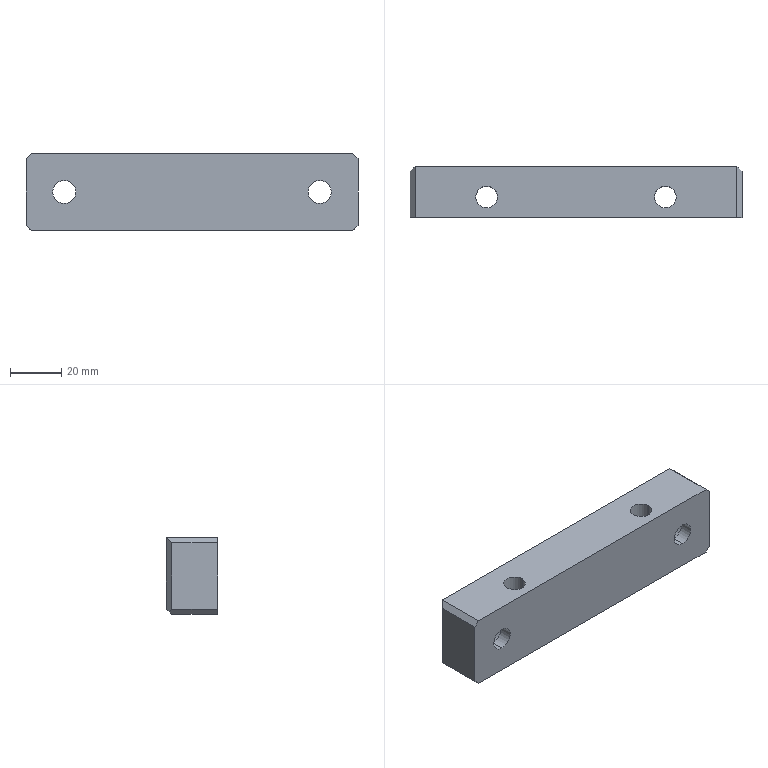Part | SolidWorks | features Chamfer 2, HoleWzd 2, Extrusion 1 | 1 solid | 27 faces | box 130 x 20 x 30 mm | volume 68135 mm3 | plane 15 | cylinder 12 | commonest cylinder face diameters 8.5 x4 9 x4 15 x4
STEP:
#1=CARTESIAN_POINT('',(-39.25,-2.,0.));
#2=VERTEX_POINT('',#1);
#3=CARTESIAN_POINT('',(-30.75,-2.,0.));
#4=VERTEX_POINT('',#3);
#5=CARTESIAN_POINT('',(-35.,-2.,0.));
#6=DIRECTION('',(0.,0.,1.));
#7=DIRECTION('',(1.,0.,0.));
#8=AXIS2_PLACEMENT_3D('',#5,#6,#7);
#9=CIRCLE('',#8,4.25);
#10=EDGE_CURVE('',#2,#4,#9,.T.);
#11=ORIENTED_EDGE('',*,*,#10,.F.);
#12=CARTESIAN_POINT('',(-39.25,-2.,30.));
#13=VERTEX_POINT('',#12);
#14=CARTESIAN_POINT('',(-39.25,-2.,30.));
#15=DIRECTION('',(0.,0.,1.));
#16=VECTOR('',#15,1000.);
#17=LINE('',#14,#16);
#18=EDGE_CURVE('',#2,#13,#17,.T.);
#19=ORIENTED_EDGE('',*,*,#18,.T.);
#20=CARTESIAN_POINT('',(-30.75,-2.,30.));
#21=VERTEX_POINT('',#20);
#22=CARTESIAN_POINT('',(-35.,-2.,30.));
#23=DIRECTION('',(0.,0.,1.));
#24=DIRECTION('',(1.,0.,0.));
#25=AXIS2_PLACEMENT_3D('',#22,#23,#24);
#26=CIRCLE('',#25,4.25);
#27=EDGE_CURVE('',#13,#21,#26,.T.);
#28=ORIENTED_EDGE('',*,*,#27,.T.);
#29=CARTESIAN_POINT('',(-30.75,-2.,30.));
#30=DIRECTION('',(0.,0.,1.));
#31=VECTOR('',#30,1000.);
#32=LINE('',#29,#31);
#33=EDGE_CURVE('',#4,#21,#32,.T.);
#34=ORIENTED_EDGE('',*,*,#33,.F.);
#35=EDGE_LOOP('',(#11,#19,#28,#34));
#36=FACE_OUTER_BOUND('',#35,.T.);
#37=CARTESIAN_POINT('',(-35.,-2.,30.));
#38=DIRECTION('',(0.,0.,1.));
#39=DIRECTION('',(1.,0.,0.));
#40=AXIS2_PLACEMENT_3D('',#37,#38,#39);
#41=CYLINDRICAL_SURFACE('',#40,4.25);
#42=ADVANCED_FACE('',(#36),#41,.F.);
#43=CARTESIAN_POINT('',(30.75,-2.,0.));
#44=VERTEX_POINT('',#43);
#45=CARTESIAN_POINT('',(39.25,-2.,0.));
#46=VERTEX_POINT('',#45);
#47=CARTESIAN_POINT('',(35.,-2.,0.));
#48=DIRECTION('',(0.,0.,1.));
#49=DIRECTION('',(1.,0.,0.));
#50=AXIS2_PLACEMENT_3D('',#47,#48,#49);
#51=CIRCLE('',#50,4.25);
#52=EDGE_CURVE('',#44,#46,#51,.T.);
#53=ORIENTED_EDGE('',*,*,#52,.F.);
#54=CARTESIAN_POINT('',(30.75,-2.,30.));
#55=VERTEX_POINT('',#54);
#56=CARTESIAN_POINT('',(30.75,-2.,30.));
#57=DIRECTION('',(0.,0.,1.));
#58=VECTOR('',#57,1000.);
#59=LINE('',#56,#58);
#60=EDGE_CURVE('',#44,#55,#59,.T.);
#61=ORIENTED_EDGE('',*,*,#60,.T.);
#62=CARTESIAN_POINT('',(39.25,-2.,30.));
#63=VERTEX_POINT('',#62);
#64=CARTESIAN_POINT('',(35.,-2.,30.));
#65=DIRECTION('',(0.,0.,1.));
#66=DIRECTION('',(1.,0.,0.));
#67=AXIS2_PLACEMENT_3D('',#64,#65,#66);
#68=CIRCLE('',#67,4.25);
#69=EDGE_CURVE('',#55,#63,#68,.T.);
#70=ORIENTED_EDGE('',*,*,#69,.T.);
#71=CARTESIAN_POINT('',(39.25,-2.,30.));
#72=DIRECTION('',(0.,0.,1.));
#73=VECTOR('',#72,1000.);
#74=LINE('',#71,#73);
#75=EDGE_CURVE('',#46,#63,#74,.T.);
#76=ORIENTED_EDGE('',*,*,#75,.F.);
#77=EDGE_LOOP('',(#53,#61,#70,#76));
#78=FACE_OUTER_BOUND('',#77,.T.);
#79=CARTESIAN_POINT('',(35.,-2.,30.));
#80=DIRECTION('',(0.,0.,1.));
#81=DIRECTION('',(1.,0.,0.));
#82=AXIS2_PLACEMENT_3D('',#79,#80,#81);
#83=CYLINDRICAL_SURFACE('',#82,4.25);
#84=ADVANCED_FACE('',(#78),#83,.F.);
#85=CARTESIAN_POINT('',(-50.,-5.,7.5));
#86=VERTEX_POINT('',#85);
#87=CARTESIAN_POINT('',(-50.,-5.,22.5));
#88=VERTEX_POINT('',#87);
#89=CARTESIAN_POINT('',(-50.,-5.,15.));
#90=DIRECTION('',(0.,1.,0.));
#91=DIRECTION('',(0.,0.,1.));
#92=AXIS2_PLACEMENT_3D('',#89,#90,#91);
#93=CIRCLE('',#92,7.5);
#94=EDGE_CURVE('',#86,#88,#93,.T.);
#95=ORIENTED_EDGE('',*,*,#94,.F.);
#96=CARTESIAN_POINT('',(-50.,10.,7.5));
#97=VERTEX_POINT('',#96);
#98=CARTESIAN_POINT('',(-50.,10.,7.5));
#99=DIRECTION('',(0.,1.,0.));
#100=VECTOR('',#99,1000.);
#101=LINE('',#98,#100);
#102=EDGE_CURVE('',#86,#97,#101,.T.);
#103=ORIENTED_EDGE('',*,*,#102,.T.);
#104=CARTESIAN_POINT('',(-50.,10.,22.5));
#105=VERTEX_POINT('',#104);
#106=CARTESIAN_POINT('',(-50.,10.,15.));
#107=DIRECTION('',(0.,1.,0.));
#108=DIRECTION('',(0.,0.,1.));
#109=AXIS2_PLACEMENT_3D('',#106,#107,#108);
#110=CIRCLE('',#109,7.5);
#111=EDGE_CURVE('',#97,#105,#110,.T.);
#112=ORIENTED_EDGE('',*,*,#111,.T.);
#113=CARTESIAN_POINT('',(-50.,10.,22.5));
#114=DIRECTION('',(0.,1.,0.));
#115=VECTOR('',#114,1000.);
#116=LINE('',#113,#115);
#117=EDGE_CURVE('',#88,#105,#116,.T.);
#118=ORIENTED_EDGE('',*,*,#117,.F.);
#119=EDGE_LOOP('',(#95,#103,#112,#118));
#120=FACE_OUTER_BOUND('',#119,.T.);
#121=CARTESIAN_POINT('',(-50.,10.,15.));
#122=DIRECTION('',(0.,1.,0.));
#123=DIRECTION('',(0.,0.,1.));
#124=AXIS2_PLACEMENT_3D('',#121,#122,#123);
#125=CYLINDRICAL_SURFACE('',#124,7.5);
#126=ADVANCED_FACE('',(#120),#125,.F.);
#127=CARTESIAN_POINT('',(-50.,-10.,10.5));
#128=VERTEX_POINT('',#127);
#129=CARTESIAN_POINT('',(-50.,-10.,19.5));
#130=VERTEX_POINT('',#129);
#131=CARTESIAN_POINT('',(-50.,-10.,15.));
#132=DIRECTION('',(0.,1.,0.));
#133=DIRECTION('',(0.,0.,1.));
#134=AXIS2_PLACEMENT_3D('',#131,#132,#133);
#135=CIRCLE('',#134,4.5);
#136=EDGE_CURVE('',#128,#130,#135,.T.);
#137=ORIENTED_EDGE('',*,*,#136,.F.);
#138=CARTESIAN_POINT('',(-50.,-5.,10.5));
#139=VERTEX_POINT('',#138);
#140=CARTESIAN_POINT('',(-50.,10.,10.5));
#141=DIRECTION('',(0.,1.,0.));
#142=VECTOR('',#141,1000.);
#143=LINE('',#140,#142);
#144=EDGE_CURVE('',#128,#139,#143,.T.);
#145=ORIENTED_EDGE('',*,*,#144,.T.);
#146=CARTESIAN_POINT('',(-50.,-5.,19.5));
#147=VERTEX_POINT('',#146);
#148=CARTESIAN_POINT('',(-50.,-5.,15.));
#149=DIRECTION('',(0.,1.,0.));
#150=DIRECTION('',(0.,0.,1.));
#151=AXIS2_PLACEMENT_3D('',#148,#149,#150);
#152=CIRCLE('',#151,4.5);
#153=EDGE_CURVE('',#139,#147,#152,.T.);
#154=ORIENTED_EDGE('',*,*,#153,.T.);
#155=CARTESIAN_POINT('',(-50.,10.,19.5));
#156=DIRECTION('',(0.,1.,0.));
#157=VECTOR('',#156,1000.);
#158=LINE('',#155,#157);
#159=EDGE_CURVE('',#130,#147,#158,.T.);
#160=ORIENTED_EDGE('',*,*,#159,.F.);
#161=EDGE_LOOP('',(#137,#145,#154,#160));
#162=FACE_OUTER_BOUND('',#161,.T.);
#163=CARTESIAN_POINT('',(-50.,10.,15.));
#164=DIRECTION('',(0.,1.,0.));
#165=DIRECTION('',(0.,0.,1.));
#166=AXIS2_PLACEMENT_3D('',#163,#164,#165);
#167=CYLINDRICAL_SURFACE('',#166,4.5);
#168=ADVANCED_FACE('',(#162),#167,.F.);
#169=CARTESIAN_POINT('',(50.,-5.,7.5));
#170=VERTEX_POINT('',#169);
#171=CARTESIAN_POINT('',(50.,-5.,22.5));
#172=VERTEX_POINT('',#171);
#173=CARTESIAN_POINT('',(50.,-5.,15.));
#174=DIRECTION('',(0.,1.,0.));
#175=DIRECTION('',(0.,0.,1.));
#176=AXIS2_PLACEMENT_3D('',#173,#174,#175);
#177=CIRCLE('',#176,7.5);
#178=EDGE_CURVE('',#170,#172,#177,.T.);
#179=ORIENTED_EDGE('',*,*,#178,.F.);
#180=CARTESIAN_POINT('',(50.,10.,7.5));
#181=VERTEX_POINT('',#180);
#182=CARTESIAN_POINT('',(50.,10.,7.5));
#183=DIRECTION('',(0.,1.,0.));
#184=VECTOR('',#183,1000.);
#185=LINE('',#182,#184);
#186=EDGE_CURVE('',#170,#181,#185,.T.);
#187=ORIENTED_EDGE('',*,*,#186,.T.);
#188=CARTESIAN_POINT('',(50.,10.,22.5));
#189=VERTEX_POINT('',#188);
#190=CARTESIAN_POINT('',(50.,10.,15.));
#191=DIRECTION('',(0.,1.,0.));
#192=DIRECTION('',(0.,0.,1.));
#193=AXIS2_PLACEMENT_3D('',#190,#191,#192);
#194=CIRCLE('',#193,7.5);
#195=EDGE_CURVE('',#181,#189,#194,.T.);
#196=ORIENTED_EDGE('',*,*,#195,.T.);
#197=CARTESIAN_POINT('',(50.,10.,22.5));
#198=DIRECTION('',(0.,1.,0.));
#199=VECTOR('',#198,1000.);
#200=LINE('',#197,#199);
#201=EDGE_CURVE('',#172,#189,#200,.T.);
#202=ORIENTED_EDGE('',*,*,#201,.F.);
#203=EDGE_LOOP('',(#179,#187,#196,#202));
#204=FACE_OUTER_BOUND('',#203,.T.);
#205=CARTESIAN_POINT('',(50.,10.,15.));
#206=DIRECTION('',(0.,1.,0.));
#207=DIRECTION('',(0.,0.,1.));
#208=AXIS2_PLACEMENT_3D('',#205,#206,#207);
#209=CYLINDRICAL_SURFACE('',#208,7.5);
#210=ADVANCED_FACE('',(#204),#209,.F.);
#211=CARTESIAN_POINT('',(50.,-10.,10.5));
#212=VERTEX_POINT('',#211);
#213=CARTESIAN_POINT('',(50.,-10.,19.5));
#214=VERTEX_POINT('',#213);
#215=CARTESIAN_POINT('',(50.,-10.,15.));
#216=DIRECTION('',(0.,1.,0.));
#217=DIRECTION('',(0.,0.,1.));
#218=AXIS2_PLACEMENT_3D('',#215,#216,#217);
#219=CIRCLE('',#218,4.5);
#220=EDGE_CURVE('',#212,#214,#219,.T.);
#221=ORIENTED_EDGE('',*,*,#220,.F.);
#222=CARTESIAN_POINT('',(50.,-5.,10.5));
#223=VERTEX_POINT('',#222);
#224=CARTESIAN_POINT('',(50.,10.,10.5));
#225=DIRECTION('',(0.,1.,0.));
#226=VECTOR('',#225,1000.);
#227=LINE('',#224,#226);
#228=EDGE_CURVE('',#212,#223,#227,.T.);
#229=ORIENTED_EDGE('',*,*,#228,.T.);
#230=CARTESIAN_POINT('',(50.,-5.,19.5));
#231=VERTEX_POINT('',#230);
#232=CARTESIAN_POINT('',(50.,-5.,15.));
#233=DIRECTION('',(0.,1.,0.));
#234=DIRECTION('',(0.,0.,1.));
#235=AXIS2_PLACEMENT_3D('',#232,#233,#234);
#236=CIRCLE('',#235,4.5);
#237=EDGE_CURVE('',#223,#231,#236,.T.);
#238=ORIENTED_EDGE('',*,*,#237,.T.);
#239=CARTESIAN_POINT('',(50.,10.,19.5));
#240=DIRECTION('',(0.,1.,0.));
#241=VECTOR('',#240,1000.);
#242=LINE('',#239,#241);
#243=EDGE_CURVE('',#214,#231,#242,.T.);
#244=ORIENTED_EDGE('',*,*,#243,.F.);
#245=EDGE_LOOP('',(#221,#229,#238,#244));
#246=FACE_OUTER_BOUND('',#245,.T.);
#247=CARTESIAN_POINT('',(50.,10.,15.));
#248=DIRECTION('',(0.,1.,0.));
#249=DIRECTION('',(0.,0.,1.));
#250=AXIS2_PLACEMENT_3D('',#247,#248,#249);
#251=CYLINDRICAL_SURFACE('',#250,4.5);
#252=ADVANCED_FACE('',(#246),#251,.F.);
#253=CARTESIAN_POINT('',(65.,-10.,28.));
#254=VERTEX_POINT('',#253);
#255=CARTESIAN_POINT('',(65.,-10.,2.));
#256=VERTEX_POINT('',#255);
#257=CARTESIAN_POINT('',(65.,-10.,30.));
#258=DIRECTION('',(0.,0.,-1.));
#259=VECTOR('',#258,1000.);
#260=LINE('',#257,#259);
#261=EDGE_CURVE('',#254,#256,#260,.T.);
#262=ORIENTED_EDGE('',*,*,#261,.T.);
#263=CARTESIAN_POINT('',(65.,8.,2.));
#264=VERTEX_POINT('',#263);
#265=CARTESIAN_POINT('',(65.,10.,2.));
#266=DIRECTION('',(0.,1.,0.));
#267=VECTOR('',#266,1000.);
#268=LINE('',#265,#267);
#269=EDGE_CURVE('',#256,#264,#268,.T.);
#270=ORIENTED_EDGE('',*,*,#269,.T.);
#271=CARTESIAN_POINT('',(65.,8.,28.));
#272=VERTEX_POINT('',#271);
#273=CARTESIAN_POINT('',(65.,8.,30.));
#274=DIRECTION('',(0.,0.,1.));
#275=VECTOR('',#274,1000.);
#276=LINE('',#273,#275);
#277=EDGE_CURVE('',#264,#272,#276,.T.);
#278=ORIENTED_EDGE('',*,*,#277,.T.);
#279=CARTESIAN_POINT('',(65.,-10.,28.));
#280=DIRECTION('',(0.,-1.,0.));
#281=VECTOR('',#280,1000.);
#282=LINE('',#279,#281);
#283=EDGE_CURVE('',#272,#254,#282,.T.);
#284=ORIENTED_EDGE('',*,*,#283,.T.);
#285=EDGE_LOOP('',(#262,#270,#278,#284));
#286=FACE_OUTER_BOUND('',#285,.T.);
#287=CARTESIAN_POINT('',(65.,10.,30.));
#288=DIRECTION('',(-1.,0.,0.));
#289=DIRECTION('',(0.,-1.,0.));
#290=AXIS2_PLACEMENT_3D('',#287,#288,#289);
#291=PLANE('',#290);
#292=ADVANCED_FACE('',(#286),#291,.F.);
#293=CARTESIAN_POINT('',(-50.,10.,15.));
#294=DIRECTION('',(0.,1.,0.));
#295=DIRECTION('',(0.,0.,1.));
#296=AXIS2_PLACEMENT_3D('',#293,#294,#295);
#297=CIRCLE('',#296,7.5);
#298=EDGE_CURVE('',#105,#97,#297,.T.);
#299=ORIENTED_EDGE('',*,*,#298,.F.);
#300=ORIENTED_EDGE('',*,*,#111,.F.);
#301=EDGE_LOOP('',(#299,#300));
#302=FACE_BOUND('',#301,.T.);
#303=CARTESIAN_POINT('',(50.,10.,15.));
#304=DIRECTION('',(0.,1.,0.));
#305=DIRECTION('',(0.,0.,1.));
#306=AXIS2_PLACEMENT_3D('',#303,#304,#305);
#307=CIRCLE('',#306,7.5);
#308=EDGE_CURVE('',#189,#181,#307,.T.);
#309=ORIENTED_EDGE('',*,*,#308,.F.);
#310=ORIENTED_EDGE('',*,*,#195,.F.);
#311=EDGE_LOOP('',(#309,#310));
#312=FACE_BOUND('',#311,.T.);
#313=CARTESIAN_POINT('',(63.,10.,30.));
#314=VERTEX_POINT('',#313);
#315=CARTESIAN_POINT('',(63.,10.,2.));
#316=VERTEX_POINT('',#315);
#317=CARTESIAN_POINT('',(63.,10.,30.));
#318=DIRECTION('',(0.,0.,-1.));
#319=VECTOR('',#318,1000.);
#320=LINE('',#317,#319);
#321=EDGE_CURVE('',#314,#316,#320,.T.);
#322=ORIENTED_EDGE('',*,*,#321,.T.);
#323=CARTESIAN_POINT('',(-63.,10.,2.));
#324=VERTEX_POINT('',#323);
#325=CARTESIAN_POINT('',(-65.,10.,2.));
#326=DIRECTION('',(-1.,0.,0.));
#327=VECTOR('',#326,1000.);
#328=LINE('',#325,#327);
#329=EDGE_CURVE('',#316,#324,#328,.T.);
#330=ORIENTED_EDGE('',*,*,#329,.T.);
#331=CARTESIAN_POINT('',(-63.,10.,30.));
#332=VERTEX_POINT('',#331);
#333=CARTESIAN_POINT('',(-63.,10.,30.));
#334=DIRECTION('',(0.,0.,1.));
#335=VECTOR('',#334,1000.);
#336=LINE('',#333,#335);
#337=EDGE_CURVE('',#324,#332,#336,.T.);
#338=ORIENTED_EDGE('',*,*,#337,.T.);
#339=CARTESIAN_POINT('',(-65.,10.,30.));
#340=DIRECTION('',(-1.,0.,0.));
#341=VECTOR('',#340,1000.);
#342=LINE('',#339,#341);
#343=EDGE_CURVE('',#314,#332,#342,.T.);
#344=ORIENTED_EDGE('',*,*,#343,.F.);
#345=EDGE_LOOP('',(#322,#330,#338,#344));
#346=FACE_OUTER_BOUND('',#345,.T.);
#347=CARTESIAN_POINT('',(-65.,10.,30.));
#348=DIRECTION('',(0.,-1.,0.));
#349=DIRECTION('',(0.,0.,-1.));
#350=AXIS2_PLACEMENT_3D('',#347,#348,#349);
#351=PLANE('',#350);
#352=ADVANCED_FACE('',(#302,#312,#346),#351,.F.);
#353=CARTESIAN_POINT('',(-65.,8.,28.));
#354=VERTEX_POINT('',#353);
#355=CARTESIAN_POINT('',(-65.,8.,2.));
#356=VERTEX_POINT('',#355);
#357=CARTESIAN_POINT('',(-65.,8.,30.));
#358=DIRECTION('',(0.,0.,-1.));
#359=VECTOR('',#358,1000.);
#360=LINE('',#357,#359);
#361=EDGE_CURVE('',#354,#356,#360,.T.);
#362=ORIENTED_EDGE('',*,*,#361,.T.);
#363=CARTESIAN_POINT('',(-65.,-10.,2.));
#364=VERTEX_POINT('',#363);
#365=CARTESIAN_POINT('',(-65.,10.,2.));
#366=DIRECTION('',(0.,-1.,0.));
#367=VECTOR('',#366,1000.);
#368=LINE('',#365,#367);
#369=EDGE_CURVE('',#356,#364,#368,.T.);
#370=ORIENTED_EDGE('',*,*,#369,.T.);
#371=CARTESIAN_POINT('',(-65.,-10.,28.));
#372=VERTEX_POINT('',#371);
#373=CARTESIAN_POINT('',(-65.,-10.,30.));
#374=DIRECTION('',(0.,0.,-1.));
#375=VECTOR('',#374,1000.);
#376=LINE('',#373,#375);
#377=EDGE_CURVE('',#372,#364,#376,.T.);
#378=ORIENTED_EDGE('',*,*,#377,.F.);
#379=CARTESIAN_POINT('',(-65.,10.,28.));
#380=DIRECTION('',(0.,1.,0.));
#381=VECTOR('',#380,1000.);
#382=LINE('',#379,#381);
#383=EDGE_CURVE('',#372,#354,#382,.T.);
#384=ORIENTED_EDGE('',*,*,#383,.T.);
#385=EDGE_LOOP('',(#362,#370,#378,#384));
#386=FACE_OUTER_BOUND('',#385,.T.);
#387=CARTESIAN_POINT('',(-65.,10.,30.));
#388=DIRECTION('',(1.,0.,0.));
#389=DIRECTION('',(0.,0.,-1.));
#390=AXIS2_PLACEMENT_3D('',#387,#388,#389);
#391=PLANE('',#390);
#392=ADVANCED_FACE('',(#386),#391,.F.);
#393=CARTESIAN_POINT('',(-50.,-10.,15.));
#394=DIRECTION('',(0.,1.,0.));
#395=DIRECTION('',(0.,0.,1.));
#396=AXIS2_PLACEMENT_3D('',#393,#394,#395);
#397=CIRCLE('',#396,4.5);
#398=EDGE_CURVE('',#130,#128,#397,.T.);
#399=ORIENTED_EDGE('',*,*,#398,.T.);
#400=ORIENTED_EDGE('',*,*,#136,.T.);
#401=EDGE_LOOP('',(#399,#400));
#402=FACE_BOUND('',#401,.T.);
#403=CARTESIAN_POINT('',(50.,-10.,15.));
#404=DIRECTION('',(0.,1.,0.));
#405=DIRECTION('',(0.,0.,1.));
#406=AXIS2_PLACEMENT_3D('',#403,#404,#405);
#407=CIRCLE('',#406,4.5);
#408=EDGE_CURVE('',#214,#212,#407,.T.);
#409=ORIENTED_EDGE('',*,*,#408,.T.);
#410=ORIENTED_EDGE('',*,*,#220,.T.);
#411=EDGE_LOOP('',(#409,#410));
#412=FACE_BOUND('',#411,.T.);
#413=ORIENTED_EDGE('',*,*,#377,.T.);
#414=CARTESIAN_POINT('',(-63.,-10.,0.));
#415=VERTEX_POINT('',#414);
#416=CARTESIAN_POINT('',(-65.,-10.,2.));
#417=DIRECTION('',(0.7071,0.,-0.7071));
#418=VECTOR('',#417,1000.);
#419=LINE('',#416,#418);
#420=EDGE_CURVE('',#364,#415,#419,.T.);
#421=ORIENTED_EDGE('',*,*,#420,.T.);
#422=CARTESIAN_POINT('',(63.,-10.,0.));
#423=VERTEX_POINT('',#422);
#424=CARTESIAN_POINT('',(-65.,-10.,0.));
#425=DIRECTION('',(1.,0.,0.));
#426=VECTOR('',#425,1000.);
#427=LINE('',#424,#426);
#428=EDGE_CURVE('',#415,#423,#427,.T.);
#429=ORIENTED_EDGE('',*,*,#428,.T.);
#430=CARTESIAN_POINT('',(65.,-10.,2.));
#431=DIRECTION('',(0.7071,0.,0.7071));
#432=VECTOR('',#431,1000.);
#433=LINE('',#430,#432);
#434=EDGE_CURVE('',#423,#256,#433,.T.);
#435=ORIENTED_EDGE('',*,*,#434,.T.);
#436=ORIENTED_EDGE('',*,*,#261,.F.);
#437=CARTESIAN_POINT('',(63.,-10.,30.));
#438=VERTEX_POINT('',#437);
#439=CARTESIAN_POINT('',(63.,-10.,30.));
#440=DIRECTION('',(-0.7071,0.,0.7071));
#441=VECTOR('',#440,1000.);
#442=LINE('',#439,#441);
#443=EDGE_CURVE('',#254,#438,#442,.T.);
#444=ORIENTED_EDGE('',*,*,#443,.T.);
#445=CARTESIAN_POINT('',(-63.,-10.,30.));
#446=VERTEX_POINT('',#445);
#447=CARTESIAN_POINT('',(-65.,-10.,30.));
#448=DIRECTION('',(1.,0.,0.));
#449=VECTOR('',#448,1000.);
#450=LINE('',#447,#449);
#451=EDGE_CURVE('',#446,#438,#450,.T.);
#452=ORIENTED_EDGE('',*,*,#451,.F.);
#453=CARTESIAN_POINT('',(-63.,-10.,30.));
#454=DIRECTION('',(-0.7071,0.,-0.7071));
#455=VECTOR('',#454,1000.);
#456=LINE('',#453,#455);
#457=EDGE_CURVE('',#446,#372,#456,.T.);
#458=ORIENTED_EDGE('',*,*,#457,.T.);
#459=EDGE_LOOP('',(#413,#421,#429,#435,#436,#444,#452,#458));
#460=FACE_OUTER_BOUND('',#459,.T.);
#461=CARTESIAN_POINT('',(-65.,-10.,30.));
#462=DIRECTION('',(0.,1.,0.));
#463=DIRECTION('',(0.,0.,1.));
#464=AXIS2_PLACEMENT_3D('',#461,#462,#463);
#465=PLANE('',#464);
#466=ADVANCED_FACE('',(#402,#412,#460),#465,.F.);
#467=CARTESIAN_POINT('',(-35.,-2.,30.));
#468=DIRECTION('',(0.,0.,1.));
#469=DIRECTION('',(1.,0.,0.));
#470=AXIS2_PLACEMENT_3D('',#467,#468,#469);
#471=CIRCLE('',#470,4.25);
#472=EDGE_CURVE('',#21,#13,#471,.T.);
#473=ORIENTED_EDGE('',*,*,#472,.F.);
#474=ORIENTED_EDGE('',*,*,#27,.F.);
#475=EDGE_LOOP('',(#473,#474));
#476=FACE_BOUND('',#475,.T.);
#477=CARTESIAN_POINT('',(35.,-2.,30.));
#478=DIRECTION('',(0.,0.,1.));
#479=DIRECTION('',(1.,0.,0.));
#480=AXIS2_PLACEMENT_3D('',#477,#478,#479);
#481=CIRCLE('',#480,4.25);
#482=EDGE_CURVE('',#63,#55,#481,.T.);
#483=ORIENTED_EDGE('',*,*,#482,.F.);
#484=ORIENTED_EDGE('',*,*,#69,.F.);
#485=EDGE_LOOP('',(#483,#484));
#486=FACE_BOUND('',#485,.T.);
#487=ORIENTED_EDGE('',*,*,#343,.T.);
#488=CARTESIAN_POINT('',(-63.,-10.,30.));
#489=DIRECTION('',(0.,-1.,0.));
#490=VECTOR('',#489,1000.);
#491=LINE('',#488,#490);
#492=EDGE_CURVE('',#332,#446,#491,.T.);
#493=ORIENTED_EDGE('',*,*,#492,.T.);
#494=ORIENTED_EDGE('',*,*,#451,.T.);
#495=CARTESIAN_POINT('',(63.,10.,30.));
#496=DIRECTION('',(0.,1.,0.));
#497=VECTOR('',#496,1000.);
#498=LINE('',#495,#497);
#499=EDGE_CURVE('',#438,#314,#498,.T.);
#500=ORIENTED_EDGE('',*,*,#499,.T.);
#501=EDGE_LOOP('',(#487,#493,#494,#500));
#502=FACE_OUTER_BOUND('',#501,.T.);
#503=CARTESIAN_POINT('',(0.,0.,30.));
#504=DIRECTION('',(0.,0.,1.));
#505=DIRECTION('',(1.,0.,0.));
#506=AXIS2_PLACEMENT_3D('',#503,#504,#505);
#507=PLANE('',#506);
#508=ADVANCED_FACE('',(#476,#486,#502),#507,.T.);
#509=CARTESIAN_POINT('',(-35.,-2.,0.));
#510=DIRECTION('',(0.,0.,1.));
#511=DIRECTION('',(1.,0.,0.));
#512=AXIS2_PLACEMENT_3D('',#509,#510,#511);
#513=CIRCLE('',#512,4.25);
#514=EDGE_CURVE('',#4,#2,#513,.T.);
#515=ORIENTED_EDGE('',*,*,#514,.T.);
#516=ORIENTED_EDGE('',*,*,#10,.T.);
#517=EDGE_LOOP('',(#515,#516));
#518=FACE_BOUND('',#517,.T.);
#519=CARTESIAN_POINT('',(35.,-2.,0.));
#520=DIRECTION('',(0.,0.,1.));
#521=DIRECTION('',(1.,0.,0.));
#522=AXIS2_PLACEMENT_3D('',#519,#520,#521);
#523=CIRCLE('',#522,4.25);
#524=EDGE_CURVE('',#46,#44,#523,.T.);
#525=ORIENTED_EDGE('',*,*,#524,.T.);
#526=ORIENTED_EDGE('',*,*,#52,.T.);
#527=EDGE_LOOP('',(#525,#526));
#528=FACE_BOUND('',#527,.T.);
#529=CARTESIAN_POINT('',(-63.,8.,0.));
#530=VERTEX_POINT('',#529);
#531=CARTESIAN_POINT('',(-63.,0.,0.));
#532=DIRECTION('',(0.,1.,0.));
#533=VECTOR('',#532,1000.);
#534=LINE('',#531,#533);
#535=EDGE_CURVE('',#415,#530,#534,.T.);
#536=ORIENTED_EDGE('',*,*,#535,.T.);
#537=CARTESIAN_POINT('',(63.,8.,0.));
#538=VERTEX_POINT('',#537);
#539=CARTESIAN_POINT('',(0.,8.,0.));
#540=DIRECTION('',(1.,0.,0.));
#541=VECTOR('',#540,1000.);
#542=LINE('',#539,#541);
#543=EDGE_CURVE('',#530,#538,#542,.T.);
#544=ORIENTED_EDGE('',*,*,#543,.T.);
#545=CARTESIAN_POINT('',(63.,0.,0.));
#546=DIRECTION('',(0.,-1.,0.));
#547=VECTOR('',#546,1000.);
#548=LINE('',#545,#547);
#549=EDGE_CURVE('',#538,#423,#548,.T.);
#550=ORIENTED_EDGE('',*,*,#549,.T.);
#551=ORIENTED_EDGE('',*,*,#428,.F.);
#552=EDGE_LOOP('',(#536,#544,#550,#551));
#553=FACE_OUTER_BOUND('',#552,.T.);
#554=CARTESIAN_POINT('',(0.,0.,0.));
#555=DIRECTION('',(0.,0.,1.));
#556=DIRECTION('',(1.,0.,0.));
#557=AXIS2_PLACEMENT_3D('',#554,#555,#556);
#558=PLANE('',#557);
#559=ADVANCED_FACE('',(#518,#528,#553),#558,.F.);
#560=ORIENTED_EDGE('',*,*,#228,.F.);
#561=ORIENTED_EDGE('',*,*,#408,.F.);
#562=ORIENTED_EDGE('',*,*,#243,.T.);
#563=CARTESIAN_POINT('',(50.,-5.,15.));
#564=DIRECTION('',(0.,1.,0.));
#565=DIRECTION('',(0.,0.,1.));
#566=AXIS2_PLACEMENT_3D('',#563,#564,#565);
#567=CIRCLE('',#566,4.5);
#568=EDGE_CURVE('',#231,#223,#567,.T.);
#569=ORIENTED_EDGE('',*,*,#568,.T.);
#570=EDGE_LOOP('',(#560,#561,#562,#569));
#571=FACE_OUTER_BOUND('',#570,.T.);
#572=CARTESIAN_POINT('',(50.,10.,15.));
#573=DIRECTION('',(0.,1.,0.));
#574=DIRECTION('',(0.,0.,1.));
#575=AXIS2_PLACEMENT_3D('',#572,#573,#574);
#576=CYLINDRICAL_SURFACE('',#575,4.5);
#577=ADVANCED_FACE('',(#571),#576,.F.);
#578=ORIENTED_EDGE('',*,*,#568,.F.);
#579=ORIENTED_EDGE('',*,*,#237,.F.);
#580=EDGE_LOOP('',(#578,#579));
#581=FACE_BOUND('',#580,.T.);
#582=CARTESIAN_POINT('',(50.,-5.,15.));
#583=DIRECTION('',(0.,1.,0.));
#584=DIRECTION('',(0.,0.,1.));
#585=AXIS2_PLACEMENT_3D('',#582,#583,#584);
#586=CIRCLE('',#585,7.5);
#587=EDGE_CURVE('',#172,#170,#586,.T.);
#588=ORIENTED_EDGE('',*,*,#587,.T.);
#589=ORIENTED_EDGE('',*,*,#178,.T.);
#590=EDGE_LOOP('',(#588,#589));
#591=FACE_OUTER_BOUND('',#590,.T.);
#592=CARTESIAN_POINT('',(54.5,-5.,15.));
#593=DIRECTION('',(0.,-1.,0.));
#594=DIRECTION('',(0.,0.,-1.));
#595=AXIS2_PLACEMENT_3D('',#592,#593,#594);
#596=PLANE('',#595);
#597=ADVANCED_FACE('',(#581,#591),#596,.F.);
#598=ORIENTED_EDGE('',*,*,#186,.F.);
#599=ORIENTED_EDGE('',*,*,#587,.F.);
#600=ORIENTED_EDGE('',*,*,#201,.T.);
#601=ORIENTED_EDGE('',*,*,#308,.T.);
#602=EDGE_LOOP('',(#598,#599,#600,#601));
#603=FACE_OUTER_BOUND('',#602,.T.);
#604=CARTESIAN_POINT('',(50.,10.,15.));
#605=DIRECTION('',(0.,1.,0.));
#606=DIRECTION('',(0.,0.,1.));
#607=AXIS2_PLACEMENT_3D('',#604,#605,#606);
#608=CYLINDRICAL_SURFACE('',#607,7.5);
#609=ADVANCED_FACE('',(#603),#608,.F.);
#610=ORIENTED_EDGE('',*,*,#144,.F.);
#611=ORIENTED_EDGE('',*,*,#398,.F.);
#612=ORIENTED_EDGE('',*,*,#159,.T.);
#613=CARTESIAN_POINT('',(-50.,-5.,15.));
#614=DIRECTION('',(0.,1.,0.));
#615=DIRECTION('',(0.,0.,1.));
#616=AXIS2_PLACEMENT_3D('',#613,#614,#615);
#617=CIRCLE('',#616,4.5);
#618=EDGE_CURVE('',#147,#139,#617,.T.);
#619=ORIENTED_EDGE('',*,*,#618,.T.);
#620=EDGE_LOOP('',(#610,#611,#612,#619));
#621=FACE_OUTER_BOUND('',#620,.T.);
#622=CARTESIAN_POINT('',(-50.,10.,15.));
#623=DIRECTION('',(0.,1.,0.));
#624=DIRECTION('',(0.,0.,1.));
#625=AXIS2_PLACEMENT_3D('',#622,#623,#624);
#626=CYLINDRICAL_SURFACE('',#625,4.5);
#627=ADVANCED_FACE('',(#621),#626,.F.);
#628=ORIENTED_EDGE('',*,*,#618,.F.);
#629=ORIENTED_EDGE('',*,*,#153,.F.);
#630=EDGE_LOOP('',(#628,#629));
#631=FACE_BOUND('',#630,.T.);
#632=CARTESIAN_POINT('',(-50.,-5.,15.));
#633=DIRECTION('',(0.,1.,0.));
#634=DIRECTION('',(0.,0.,1.));
#635=AXIS2_PLACEMENT_3D('',#632,#633,#634);
#636=CIRCLE('',#635,7.5);
#637=EDGE_CURVE('',#88,#86,#636,.T.);
#638=ORIENTED_EDGE('',*,*,#637,.T.);
#639=ORIENTED_EDGE('',*,*,#94,.T.);
#640=EDGE_LOOP('',(#638,#639));
#641=FACE_OUTER_BOUND('',#640,.T.);
#642=CARTESIAN_POINT('',(-45.5,-5.,15.));
#643=DIRECTION('',(0.,-1.,0.));
#644=DIRECTION('',(0.,0.,-1.));
#645=AXIS2_PLACEMENT_3D('',#642,#643,#644);
#646=PLANE('',#645);
#647=ADVANCED_FACE('',(#631,#641),#646,.F.);
#648=ORIENTED_EDGE('',*,*,#102,.F.);
#649=ORIENTED_EDGE('',*,*,#637,.F.);
#650=ORIENTED_EDGE('',*,*,#117,.T.);
#651=ORIENTED_EDGE('',*,*,#298,.T.);
#652=EDGE_LOOP('',(#648,#649,#650,#651));
#653=FACE_OUTER_BOUND('',#652,.T.);
#654=CARTESIAN_POINT('',(-50.,10.,15.));
#655=DIRECTION('',(0.,1.,0.));
#656=DIRECTION('',(0.,0.,1.));
#657=AXIS2_PLACEMENT_3D('',#654,#655,#656);
#658=CYLINDRICAL_SURFACE('',#657,7.5);
#659=ADVANCED_FACE('',(#653),#658,.F.);
#660=ORIENTED_EDGE('',*,*,#60,.F.);
#661=ORIENTED_EDGE('',*,*,#524,.F.);
#662=ORIENTED_EDGE('',*,*,#75,.T.);
#663=ORIENTED_EDGE('',*,*,#482,.T.);
#664=EDGE_LOOP('',(#660,#661,#662,#663));
#665=FACE_OUTER_BOUND('',#664,.T.);
#666=CARTESIAN_POINT('',(35.,-2.,30.));
#667=DIRECTION('',(0.,0.,1.));
#668=DIRECTION('',(1.,0.,0.));
#669=AXIS2_PLACEMENT_3D('',#666,#667,#668);
#670=CYLINDRICAL_SURFACE('',#669,4.25);
#671=ADVANCED_FACE('',(#665),#670,.F.);
#672=ORIENTED_EDGE('',*,*,#18,.F.);
#673=ORIENTED_EDGE('',*,*,#514,.F.);
#674=ORIENTED_EDGE('',*,*,#33,.T.);
#675=ORIENTED_EDGE('',*,*,#472,.T.);
#676=EDGE_LOOP('',(#672,#673,#674,#675));
#677=FACE_OUTER_BOUND('',#676,.T.);
#678=CARTESIAN_POINT('',(-35.,-2.,30.));
#679=DIRECTION('',(0.,0.,1.));
#680=DIRECTION('',(1.,0.,0.));
#681=AXIS2_PLACEMENT_3D('',#678,#679,#680);
#682=CYLINDRICAL_SURFACE('',#681,4.25);
#683=ADVANCED_FACE('',(#677),#682,.F.);
#684=ORIENTED_EDGE('',*,*,#457,.F.);
#685=ORIENTED_EDGE('',*,*,#492,.F.);
#686=CARTESIAN_POINT('',(-66.333,6.667,26.667));
#687=DIRECTION('',(0.5774,0.5774,0.5774));
#688=VECTOR('',#687,1000.);
#689=LINE('',#686,#688);
#690=EDGE_CURVE('',#354,#332,#689,.T.);
#691=ORIENTED_EDGE('',*,*,#690,.F.);
#692=ORIENTED_EDGE('',*,*,#383,.F.);
#693=EDGE_LOOP('',(#684,#685,#691,#692));
#694=FACE_OUTER_BOUND('',#693,.T.);
#695=CARTESIAN_POINT('',(-63.,0.,30.));
#696=DIRECTION('',(-0.7071,0.,0.7071));
#697=DIRECTION('',(0.,1.,0.));
#698=AXIS2_PLACEMENT_3D('',#695,#696,#697);
#699=PLANE('',#698);
#700=ADVANCED_FACE('',(#694),#699,.T.);
#701=ORIENTED_EDGE('',*,*,#337,.F.);
#702=CARTESIAN_POINT('',(-64.,9.,1.));
#703=VERTEX_POINT('',#702);
#704=CARTESIAN_POINT('',(-55.,18.,10.));
#705=DIRECTION('',(-0.5774,-0.5774,-0.5774));
#706=VECTOR('',#705,1000.);
#707=LINE('',#704,#706);
#708=EDGE_CURVE('',#324,#703,#707,.T.);
#709=ORIENTED_EDGE('',*,*,#708,.T.);
#710=CARTESIAN_POINT('',(-74.333,-1.333,11.333));
#711=DIRECTION('',(0.5774,0.5774,-0.5774));
#712=VECTOR('',#711,1000.);
#713=LINE('',#710,#712);
#714=EDGE_CURVE('',#356,#703,#713,.T.);
#715=ORIENTED_EDGE('',*,*,#714,.F.);
#716=ORIENTED_EDGE('',*,*,#361,.F.);
#717=ORIENTED_EDGE('',*,*,#690,.T.);
#718=EDGE_LOOP('',(#701,#709,#715,#716,#717));
#719=FACE_OUTER_BOUND('',#718,.T.);
#720=CARTESIAN_POINT('',(-65.,8.,30.));
#721=DIRECTION('',(0.7071,-0.7071,0.));
#722=DIRECTION('',(0.,0.,-1.));
#723=AXIS2_PLACEMENT_3D('',#720,#721,#722);
#724=PLANE('',#723);
#725=ADVANCED_FACE('',(#719),#724,.F.);
#726=ORIENTED_EDGE('',*,*,#714,.T.);
#727=CARTESIAN_POINT('',(-65.,10.,2.));
#728=DIRECTION('',(0.5774,-0.5774,-0.5774));
#729=VECTOR('',#728,1000.);
#730=LINE('',#727,#729);
#731=EDGE_CURVE('',#703,#530,#730,.T.);
#732=ORIENTED_EDGE('',*,*,#731,.T.);
#733=ORIENTED_EDGE('',*,*,#535,.F.);
#734=ORIENTED_EDGE('',*,*,#420,.F.);
#735=ORIENTED_EDGE('',*,*,#369,.F.);
#736=EDGE_LOOP('',(#726,#732,#733,#734,#735));
#737=FACE_OUTER_BOUND('',#736,.T.);
#738=CARTESIAN_POINT('',(-65.,10.,2.));
#739=DIRECTION('',(0.7071,0.,0.7071));
#740=DIRECTION('',(0.,-1.,0.));
#741=AXIS2_PLACEMENT_3D('',#738,#739,#740);
#742=PLANE('',#741);
#743=ADVANCED_FACE('',(#737),#742,.F.);
#744=ORIENTED_EDGE('',*,*,#443,.F.);
#745=ORIENTED_EDGE('',*,*,#283,.F.);
#746=CARTESIAN_POINT('',(66.333,6.667,26.667));
#747=DIRECTION('',(0.5774,-0.5774,-0.5774));
#748=VECTOR('',#747,1000.);
#749=LINE('',#746,#748);
#750=EDGE_CURVE('',#314,#272,#749,.T.);
#751=ORIENTED_EDGE('',*,*,#750,.F.);
#752=ORIENTED_EDGE('',*,*,#499,.F.);
#753=EDGE_LOOP('',(#744,#745,#751,#752));
#754=FACE_OUTER_BOUND('',#753,.T.);
#755=CARTESIAN_POINT('',(63.,0.,30.));
#756=DIRECTION('',(0.7071,0.,0.7071));
#757=DIRECTION('',(0.,-1.,0.));
#758=AXIS2_PLACEMENT_3D('',#755,#756,#757);
#759=PLANE('',#758);
#760=ADVANCED_FACE('',(#754),#759,.T.);
#761=CARTESIAN_POINT('',(64.,9.,1.));
#762=VERTEX_POINT('',#761);
#763=CARTESIAN_POINT('',(73.,0.,10.));
#764=DIRECTION('',(0.5774,-0.5774,0.5774));
#765=VECTOR('',#764,1000.);
#766=LINE('',#763,#765);
#767=EDGE_CURVE('',#762,#264,#766,.T.);
#768=ORIENTED_EDGE('',*,*,#767,.F.);
#769=CARTESIAN_POINT('',(53.667,19.333,11.333));
#770=DIRECTION('',(-0.5774,0.5774,0.5774));
#771=VECTOR('',#770,1000.);
#772=LINE('',#769,#771);
#773=EDGE_CURVE('',#762,#316,#772,.T.);
#774=ORIENTED_EDGE('',*,*,#773,.T.);
#775=ORIENTED_EDGE('',*,*,#321,.F.);
#776=ORIENTED_EDGE('',*,*,#750,.T.);
#777=ORIENTED_EDGE('',*,*,#277,.F.);
#778=EDGE_LOOP('',(#768,#774,#775,#776,#777));
#779=FACE_OUTER_BOUND('',#778,.T.);
#780=CARTESIAN_POINT('',(63.,10.,30.));
#781=DIRECTION('',(-0.7071,-0.7071,0.));
#782=DIRECTION('',(0.,0.,-1.));
#783=AXIS2_PLACEMENT_3D('',#780,#781,#782);
#784=PLANE('',#783);
#785=ADVANCED_FACE('',(#779),#784,.F.);
#786=ORIENTED_EDGE('',*,*,#549,.F.);
#787=CARTESIAN_POINT('',(65.,10.,2.));
#788=DIRECTION('',(0.5774,0.5774,0.5774));
#789=VECTOR('',#788,1000.);
#790=LINE('',#787,#789);
#791=EDGE_CURVE('',#538,#762,#790,.T.);
#792=ORIENTED_EDGE('',*,*,#791,.T.);
#793=ORIENTED_EDGE('',*,*,#767,.T.);
#794=ORIENTED_EDGE('',*,*,#269,.F.);
#795=ORIENTED_EDGE('',*,*,#434,.F.);
#796=EDGE_LOOP('',(#786,#792,#793,#794,#795));
#797=FACE_OUTER_BOUND('',#796,.T.);
#798=CARTESIAN_POINT('',(65.,10.,2.));
#799=DIRECTION('',(-0.7071,0.,0.7071));
#800=DIRECTION('',(0.,1.,0.));
#801=AXIS2_PLACEMENT_3D('',#798,#799,#800);
#802=PLANE('',#801);
#803=ADVANCED_FACE('',(#797),#802,.F.);
#804=ORIENTED_EDGE('',*,*,#791,.F.);
#805=ORIENTED_EDGE('',*,*,#543,.F.);
#806=ORIENTED_EDGE('',*,*,#731,.F.);
#807=ORIENTED_EDGE('',*,*,#708,.F.);
#808=ORIENTED_EDGE('',*,*,#329,.F.);
#809=ORIENTED_EDGE('',*,*,#773,.F.);
#810=EDGE_LOOP('',(#804,#805,#806,#807,#808,#809));
#811=FACE_OUTER_BOUND('',#810,.T.);
#812=CARTESIAN_POINT('',(-65.,10.,2.));
#813=DIRECTION('',(0.,-0.7071,0.7071));
#814=DIRECTION('',(-1.,0.,0.));
#815=AXIS2_PLACEMENT_3D('',#812,#813,#814);
#816=PLANE('',#815);
#817=ADVANCED_FACE('',(#811),#816,.F.);
#818=CLOSED_SHELL('',(#42,#84,#126,#168,#210,#252,#292,#352,#392,#466,#508,#559,#577,#597,#609,#627,#647,#659,#671,#683,#700,#725,#743,#760,#785,#803,#817));
#819=MANIFOLD_SOLID_BREP('',#818);
#820=CARTESIAN_POINT('',(0.,0.,0.));
#821=DIRECTION('',(0.,0.,1.));
#822=DIRECTION('',(1.,0.,0.));
#823=AXIS2_PLACEMENT_3D('',#820,#821,#822);
#824=(LENGTH_UNIT()NAMED_UNIT(*)SI_UNIT(.MILLI.,.METRE.));
#825=UNCERTAINTY_MEASURE_WITH_UNIT(LENGTH_MEASURE(0.00001),#824,'','');
#826=(NAMED_UNIT(*)PLANE_ANGLE_UNIT()SI_UNIT($,.RADIAN.));
#827=(NAMED_UNIT(*)SI_UNIT($,.STERADIAN.)SOLID_ANGLE_UNIT());
#828=(GEOMETRIC_REPRESENTATION_CONTEXT(3)GLOBAL_UNCERTAINTY_ASSIGNED_CONTEXT((#825))GLOBAL_UNIT_ASSIGNED_CONTEXT((#824,#826,#827))REPRESENTATION_CONTEXT('',''));
#829=ADVANCED_BREP_SHAPE_REPRESENTATION('',(#819,#823),#828);